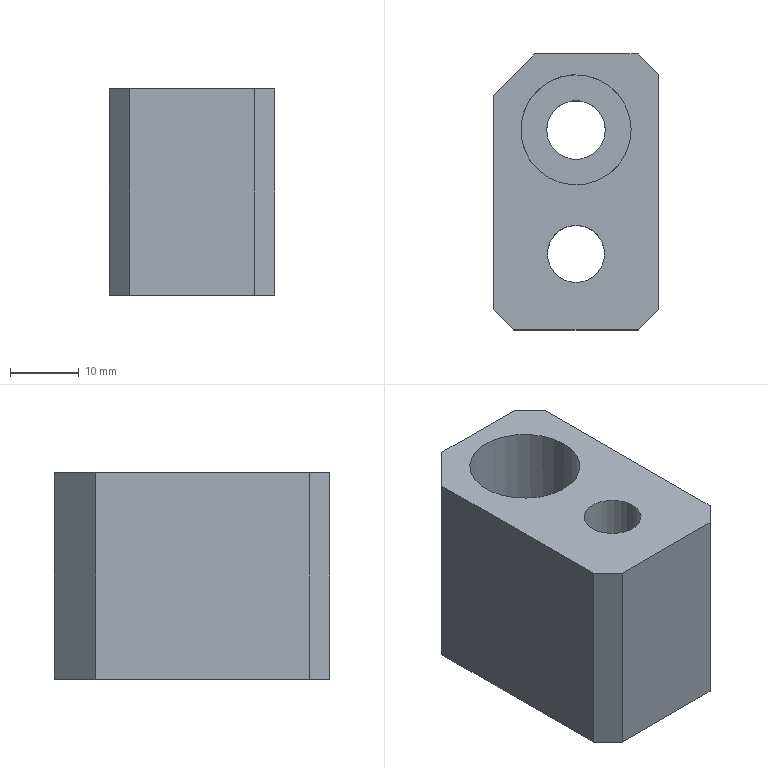Part | NX | features LIN_SOLID_COLOR 2 | 1 solid | 14 faces | box 24 x 40 x 30 mm | volume 22365 mm3 | plane 11 | cylinder 3 | commonest cylinder face diameters 8.3 x1 8.5 x1 16 x1
STEP:
#1=CARTESIAN_POINT('',(-225.,-65.,-31.5));
#2=VERTEX_POINT('',#1);
#3=CARTESIAN_POINT('',(-225.,-96.,-31.5));
#4=VERTEX_POINT('',#3);
#5=CARTESIAN_POINT('',(-225.,-81.,-31.5));
#6=DIRECTION('',(0.,-1.,0.));
#7=VECTOR('',#6,1000.);
#8=LINE('',#5,#7);
#9=EDGE_CURVE('',#2,#4,#8,.T.);
#10=ORIENTED_EDGE('',*,*,#9,.F.);
#11=CARTESIAN_POINT('',(-219.,-59.,-31.5));
#12=VERTEX_POINT('',#11);
#13=CARTESIAN_POINT('',(-227.,-67.,-31.5));
#14=DIRECTION('',(-0.7071,-0.7071,0.));
#15=VECTOR('',#14,1000.);
#16=LINE('',#13,#15);
#17=EDGE_CURVE('',#2,#12,#16,.F.);
#18=ORIENTED_EDGE('',*,*,#17,.T.);
#19=CARTESIAN_POINT('',(-204.,-59.,-31.5));
#20=VERTEX_POINT('',#19);
#21=CARTESIAN_POINT('',(-213.,-59.,-31.5));
#22=DIRECTION('',(-1.,0.,0.));
#23=VECTOR('',#22,1000.);
#24=LINE('',#21,#23);
#25=EDGE_CURVE('',#20,#12,#24,.T.);
#26=ORIENTED_EDGE('',*,*,#25,.F.);
#27=CARTESIAN_POINT('',(-201.,-62.,-31.5));
#28=VERTEX_POINT('',#27);
#29=CARTESIAN_POINT('',(-197.5,-65.5,-31.5));
#30=DIRECTION('',(-0.7071,0.7071,0.));
#31=VECTOR('',#30,1000.);
#32=LINE('',#29,#31);
#33=EDGE_CURVE('',#20,#28,#32,.F.);
#34=ORIENTED_EDGE('',*,*,#33,.T.);
#35=CARTESIAN_POINT('',(-201.,-96.,-31.5));
#36=VERTEX_POINT('',#35);
#37=CARTESIAN_POINT('',(-201.,-81.,-31.5));
#38=DIRECTION('',(0.,1.,0.));
#39=VECTOR('',#38,1000.);
#40=LINE('',#37,#39);
#41=EDGE_CURVE('',#36,#28,#40,.T.);
#42=ORIENTED_EDGE('',*,*,#41,.F.);
#43=CARTESIAN_POINT('',(-204.,-99.,-31.5));
#44=VERTEX_POINT('',#43);
#45=CARTESIAN_POINT('',(-199.5,-94.5,-31.5));
#46=DIRECTION('',(0.7071,0.7071,0.));
#47=VECTOR('',#46,1000.);
#48=LINE('',#45,#47);
#49=EDGE_CURVE('',#36,#44,#48,.F.);
#50=ORIENTED_EDGE('',*,*,#49,.T.);
#51=CARTESIAN_POINT('',(-222.,-99.,-31.5));
#52=VERTEX_POINT('',#51);
#53=CARTESIAN_POINT('',(-213.,-99.,-31.5));
#54=DIRECTION('',(1.,0.,0.));
#55=VECTOR('',#54,1000.);
#56=LINE('',#53,#55);
#57=EDGE_CURVE('',#52,#44,#56,.T.);
#58=ORIENTED_EDGE('',*,*,#57,.F.);
#59=CARTESIAN_POINT('',(-226.5,-94.5,-31.5));
#60=DIRECTION('',(0.7071,-0.7071,0.));
#61=VECTOR('',#60,1000.);
#62=LINE('',#59,#61);
#63=EDGE_CURVE('',#52,#4,#62,.F.);
#64=ORIENTED_EDGE('',*,*,#63,.T.);
#65=EDGE_LOOP('',(#10,#18,#26,#34,#42,#50,#58,#64));
#66=FACE_BOUND('',#65,.T.);
#67=CARTESIAN_POINT('',(-208.85,-88.,-31.5));
#68=VERTEX_POINT('',#67);
#69=CARTESIAN_POINT('',(-213.,-88.,-31.5));
#70=DIRECTION('',(0.,0.,-1.));
#71=DIRECTION('',(1.,0.,0.));
#72=AXIS2_PLACEMENT_3D('',#69,#70,#71);
#73=CIRCLE('',#72,4.15);
#74=EDGE_CURVE('',#68,#68,#73,.T.);
#75=ORIENTED_EDGE('',*,*,#74,.F.);
#76=EDGE_LOOP('',(#75));
#77=FACE_BOUND('',#76,.T.);
#78=CARTESIAN_POINT('',(-217.25,-70.,-31.5));
#79=VERTEX_POINT('',#78);
#80=CARTESIAN_POINT('',(-213.,-70.,-31.5));
#81=DIRECTION('',(0.,0.,-1.));
#82=DIRECTION('',(-1.,0.,0.));
#83=AXIS2_PLACEMENT_3D('',#80,#81,#82);
#84=CIRCLE('',#83,4.25);
#85=EDGE_CURVE('',#79,#79,#84,.F.);
#86=ORIENTED_EDGE('',*,*,#85,.T.);
#87=EDGE_LOOP('',(#86));
#88=FACE_BOUND('',#87,.T.);
#89=CARTESIAN_POINT('',(-213.,-81.,-31.5));
#90=DIRECTION('',(0.,0.,-1.));
#91=DIRECTION('',(0.,-1.,0.));
#92=AXIS2_PLACEMENT_3D('',#89,#90,#91);
#93=PLANE('',#92);
#94=ADVANCED_FACE('',(#66,#77,#88),#93,.T.);
#95=CARTESIAN_POINT('',(-205.,-70.,-1.5));
#96=VERTEX_POINT('',#95);
#97=CARTESIAN_POINT('',(-213.,-70.,-1.5));
#98=DIRECTION('',(0.,0.,1.));
#99=DIRECTION('',(1.,0.,0.));
#100=AXIS2_PLACEMENT_3D('',#97,#98,#99);
#101=CIRCLE('',#100,8.);
#102=EDGE_CURVE('',#96,#96,#101,.T.);
#103=ORIENTED_EDGE('',*,*,#102,.F.);
#104=EDGE_LOOP('',(#103));
#105=FACE_BOUND('',#104,.T.);
#106=CARTESIAN_POINT('',(-217.15,-88.,-1.5));
#107=VERTEX_POINT('',#106);
#108=CARTESIAN_POINT('',(-213.,-88.,-1.5));
#109=DIRECTION('',(0.,0.,1.));
#110=DIRECTION('',(-1.,0.,0.));
#111=AXIS2_PLACEMENT_3D('',#108,#109,#110);
#112=CIRCLE('',#111,4.15);
#113=EDGE_CURVE('',#107,#107,#112,.T.);
#114=ORIENTED_EDGE('',*,*,#113,.F.);
#115=EDGE_LOOP('',(#114));
#116=FACE_BOUND('',#115,.T.);
#117=CARTESIAN_POINT('',(-219.,-59.,-1.5));
#118=VERTEX_POINT('',#117);
#119=CARTESIAN_POINT('',(-204.,-59.,-1.5));
#120=VERTEX_POINT('',#119);
#121=CARTESIAN_POINT('',(-213.,-59.,-1.5));
#122=DIRECTION('',(1.,0.,0.));
#123=VECTOR('',#122,1000.);
#124=LINE('',#121,#123);
#125=EDGE_CURVE('',#118,#120,#124,.T.);
#126=ORIENTED_EDGE('',*,*,#125,.F.);
#127=CARTESIAN_POINT('',(-225.,-65.,-1.5));
#128=VERTEX_POINT('',#127);
#129=CARTESIAN_POINT('',(-227.,-67.,-1.5));
#130=DIRECTION('',(0.7071,0.7071,0.));
#131=VECTOR('',#130,1000.);
#132=LINE('',#129,#131);
#133=EDGE_CURVE('',#118,#128,#132,.F.);
#134=ORIENTED_EDGE('',*,*,#133,.T.);
#135=CARTESIAN_POINT('',(-225.,-96.,-1.5));
#136=VERTEX_POINT('',#135);
#137=CARTESIAN_POINT('',(-225.,-81.,-1.5));
#138=DIRECTION('',(0.,1.,0.));
#139=VECTOR('',#138,1000.);
#140=LINE('',#137,#139);
#141=EDGE_CURVE('',#136,#128,#140,.T.);
#142=ORIENTED_EDGE('',*,*,#141,.F.);
#143=CARTESIAN_POINT('',(-222.,-99.,-1.5));
#144=VERTEX_POINT('',#143);
#145=CARTESIAN_POINT('',(-226.5,-94.5,-1.5));
#146=DIRECTION('',(-0.7071,0.7071,0.));
#147=VECTOR('',#146,1000.);
#148=LINE('',#145,#147);
#149=EDGE_CURVE('',#136,#144,#148,.F.);
#150=ORIENTED_EDGE('',*,*,#149,.T.);
#151=CARTESIAN_POINT('',(-204.,-99.,-1.5));
#152=VERTEX_POINT('',#151);
#153=CARTESIAN_POINT('',(-213.,-99.,-1.5));
#154=DIRECTION('',(-1.,0.,0.));
#155=VECTOR('',#154,1000.);
#156=LINE('',#153,#155);
#157=EDGE_CURVE('',#152,#144,#156,.T.);
#158=ORIENTED_EDGE('',*,*,#157,.F.);
#159=CARTESIAN_POINT('',(-201.,-96.,-1.5));
#160=VERTEX_POINT('',#159);
#161=CARTESIAN_POINT('',(-199.5,-94.5,-1.5));
#162=DIRECTION('',(-0.7071,-0.7071,0.));
#163=VECTOR('',#162,1000.);
#164=LINE('',#161,#163);
#165=EDGE_CURVE('',#152,#160,#164,.F.);
#166=ORIENTED_EDGE('',*,*,#165,.T.);
#167=CARTESIAN_POINT('',(-201.,-62.,-1.5));
#168=VERTEX_POINT('',#167);
#169=CARTESIAN_POINT('',(-201.,-81.,-1.5));
#170=DIRECTION('',(0.,-1.,0.));
#171=VECTOR('',#170,1000.);
#172=LINE('',#169,#171);
#173=EDGE_CURVE('',#168,#160,#172,.T.);
#174=ORIENTED_EDGE('',*,*,#173,.F.);
#175=CARTESIAN_POINT('',(-197.5,-65.5,-1.5));
#176=DIRECTION('',(0.7071,-0.7071,0.));
#177=VECTOR('',#176,1000.);
#178=LINE('',#175,#177);
#179=EDGE_CURVE('',#168,#120,#178,.F.);
#180=ORIENTED_EDGE('',*,*,#179,.T.);
#181=EDGE_LOOP('',(#126,#134,#142,#150,#158,#166,#174,#180));
#182=FACE_BOUND('',#181,.T.);
#183=CARTESIAN_POINT('',(-213.,-81.,-1.5));
#184=DIRECTION('',(0.,0.,1.));
#185=DIRECTION('',(0.,1.,0.));
#186=AXIS2_PLACEMENT_3D('',#183,#184,#185);
#187=PLANE('',#186);
#188=ADVANCED_FACE('',(#105,#116,#182),#187,.T.);
#189=ORIENTED_EDGE('',*,*,#41,.T.);
#190=CARTESIAN_POINT('',(-201.,-62.,-31.5));
#191=DIRECTION('',(0.,0.,1.));
#192=VECTOR('',#191,1000.);
#193=LINE('',#190,#192);
#194=EDGE_CURVE('',#28,#168,#193,.T.);
#195=ORIENTED_EDGE('',*,*,#194,.T.);
#196=ORIENTED_EDGE('',*,*,#173,.T.);
#197=CARTESIAN_POINT('',(-201.,-96.,-31.5));
#198=DIRECTION('',(0.,0.,-1.));
#199=VECTOR('',#198,1000.);
#200=LINE('',#197,#199);
#201=EDGE_CURVE('',#160,#36,#200,.T.);
#202=ORIENTED_EDGE('',*,*,#201,.T.);
#203=EDGE_LOOP('',(#189,#195,#196,#202));
#204=FACE_BOUND('',#203,.T.);
#205=CARTESIAN_POINT('',(-201.,-81.,-31.5));
#206=DIRECTION('',(1.,0.,0.));
#207=DIRECTION('',(0.,0.,-1.));
#208=AXIS2_PLACEMENT_3D('',#205,#206,#207);
#209=PLANE('',#208);
#210=ADVANCED_FACE('',(#204),#209,.T.);
#211=ORIENTED_EDGE('',*,*,#157,.T.);
#212=CARTESIAN_POINT('',(-222.,-99.,-31.5));
#213=DIRECTION('',(0.,0.,-1.));
#214=VECTOR('',#213,1000.);
#215=LINE('',#212,#214);
#216=EDGE_CURVE('',#144,#52,#215,.T.);
#217=ORIENTED_EDGE('',*,*,#216,.T.);
#218=ORIENTED_EDGE('',*,*,#57,.T.);
#219=CARTESIAN_POINT('',(-204.,-99.,-31.5));
#220=DIRECTION('',(0.,0.,1.));
#221=VECTOR('',#220,1000.);
#222=LINE('',#219,#221);
#223=EDGE_CURVE('',#44,#152,#222,.T.);
#224=ORIENTED_EDGE('',*,*,#223,.T.);
#225=EDGE_LOOP('',(#211,#217,#218,#224));
#226=FACE_BOUND('',#225,.T.);
#227=CARTESIAN_POINT('',(-213.,-99.,-31.5));
#228=DIRECTION('',(0.,-1.,0.));
#229=DIRECTION('',(0.,0.,1.));
#230=AXIS2_PLACEMENT_3D('',#227,#228,#229);
#231=PLANE('',#230);
#232=ADVANCED_FACE('',(#226),#231,.T.);
#233=ORIENTED_EDGE('',*,*,#141,.T.);
#234=CARTESIAN_POINT('',(-225.,-65.,-31.5));
#235=DIRECTION('',(0.,0.,-1.));
#236=VECTOR('',#235,1000.);
#237=LINE('',#234,#236);
#238=EDGE_CURVE('',#128,#2,#237,.T.);
#239=ORIENTED_EDGE('',*,*,#238,.T.);
#240=ORIENTED_EDGE('',*,*,#9,.T.);
#241=CARTESIAN_POINT('',(-225.,-96.,-31.5));
#242=DIRECTION('',(0.,0.,1.));
#243=VECTOR('',#242,1000.);
#244=LINE('',#241,#243);
#245=EDGE_CURVE('',#4,#136,#244,.T.);
#246=ORIENTED_EDGE('',*,*,#245,.T.);
#247=EDGE_LOOP('',(#233,#239,#240,#246));
#248=FACE_BOUND('',#247,.T.);
#249=CARTESIAN_POINT('',(-225.,-81.,-31.5));
#250=DIRECTION('',(-1.,0.,0.));
#251=DIRECTION('',(0.,0.,1.));
#252=AXIS2_PLACEMENT_3D('',#249,#250,#251);
#253=PLANE('',#252);
#254=ADVANCED_FACE('',(#248),#253,.T.);
#255=ORIENTED_EDGE('',*,*,#25,.T.);
#256=CARTESIAN_POINT('',(-219.,-59.,-31.5));
#257=DIRECTION('',(0.,0.,1.));
#258=VECTOR('',#257,1000.);
#259=LINE('',#256,#258);
#260=EDGE_CURVE('',#12,#118,#259,.T.);
#261=ORIENTED_EDGE('',*,*,#260,.T.);
#262=ORIENTED_EDGE('',*,*,#125,.T.);
#263=CARTESIAN_POINT('',(-204.,-59.,-31.5));
#264=DIRECTION('',(0.,0.,-1.));
#265=VECTOR('',#264,1000.);
#266=LINE('',#263,#265);
#267=EDGE_CURVE('',#120,#20,#266,.T.);
#268=ORIENTED_EDGE('',*,*,#267,.T.);
#269=EDGE_LOOP('',(#255,#261,#262,#268));
#270=FACE_BOUND('',#269,.T.);
#271=CARTESIAN_POINT('',(-213.,-59.,-31.5));
#272=DIRECTION('',(0.,1.,0.));
#273=DIRECTION('',(0.,0.,-1.));
#274=AXIS2_PLACEMENT_3D('',#271,#272,#273);
#275=PLANE('',#274);
#276=ADVANCED_FACE('',(#270),#275,.T.);
#277=ORIENTED_EDGE('',*,*,#113,.T.);
#278=EDGE_LOOP('',(#277));
#279=FACE_BOUND('',#278,.T.);
#280=ORIENTED_EDGE('',*,*,#74,.T.);
#281=EDGE_LOOP('',(#280));
#282=FACE_BOUND('',#281,.T.);
#283=CARTESIAN_POINT('',(-213.,-88.,-66.5));
#284=DIRECTION('',(0.,0.,1.));
#285=DIRECTION('',(0.,1.,0.));
#286=AXIS2_PLACEMENT_3D('',#283,#284,#285);
#287=CYLINDRICAL_SURFACE('',#286,4.15);
#288=ADVANCED_FACE('',(#279,#282),#287,.F.);
#289=CARTESIAN_POINT('',(-217.25,-70.,-16.5));
#290=VERTEX_POINT('',#289);
#291=CARTESIAN_POINT('',(-213.,-70.,-16.5));
#292=DIRECTION('',(0.,0.,-1.));
#293=DIRECTION('',(-1.,0.,0.));
#294=AXIS2_PLACEMENT_3D('',#291,#292,#293);
#295=CIRCLE('',#294,4.25);
#296=EDGE_CURVE('',#290,#290,#295,.F.);
#297=ORIENTED_EDGE('',*,*,#296,.T.);
#298=EDGE_LOOP('',(#297));
#299=FACE_BOUND('',#298,.T.);
#300=ORIENTED_EDGE('',*,*,#85,.F.);
#301=EDGE_LOOP('',(#300));
#302=FACE_BOUND('',#301,.T.);
#303=CARTESIAN_POINT('',(-213.,-70.,-31.5));
#304=DIRECTION('',(0.,0.,1.));
#305=DIRECTION('',(0.,1.,0.));
#306=AXIS2_PLACEMENT_3D('',#303,#304,#305);
#307=CYLINDRICAL_SURFACE('',#306,4.25);
#308=ADVANCED_FACE('',(#299,#302),#307,.F.);
#309=CARTESIAN_POINT('',(-221.,-70.,-16.5));
#310=VERTEX_POINT('',#309);
#311=CARTESIAN_POINT('',(-213.,-70.,-16.5));
#312=DIRECTION('',(0.,0.,-1.));
#313=DIRECTION('',(-1.,0.,0.));
#314=AXIS2_PLACEMENT_3D('',#311,#312,#313);
#315=CIRCLE('',#314,8.);
#316=EDGE_CURVE('',#310,#310,#315,.T.);
#317=ORIENTED_EDGE('',*,*,#316,.F.);
#318=EDGE_LOOP('',(#317));
#319=FACE_BOUND('',#318,.T.);
#320=ORIENTED_EDGE('',*,*,#296,.F.);
#321=EDGE_LOOP('',(#320));
#322=FACE_BOUND('',#321,.T.);
#323=CARTESIAN_POINT('',(-213.,-70.,-16.5));
#324=DIRECTION('',(0.,0.,-1.));
#325=DIRECTION('',(0.,-1.,0.));
#326=AXIS2_PLACEMENT_3D('',#323,#324,#325);
#327=PLANE('',#326);
#328=ADVANCED_FACE('',(#319,#322),#327,.F.);
#329=ORIENTED_EDGE('',*,*,#102,.T.);
#330=EDGE_LOOP('',(#329));
#331=FACE_BOUND('',#330,.T.);
#332=ORIENTED_EDGE('',*,*,#316,.T.);
#333=EDGE_LOOP('',(#332));
#334=FACE_BOUND('',#333,.T.);
#335=CARTESIAN_POINT('',(-213.,-70.,-11.5));
#336=DIRECTION('',(0.,0.,1.));
#337=DIRECTION('',(0.,1.,0.));
#338=AXIS2_PLACEMENT_3D('',#335,#336,#337);
#339=CYLINDRICAL_SURFACE('',#338,8.);
#340=ADVANCED_FACE('',(#331,#334),#339,.F.);
#341=ORIENTED_EDGE('',*,*,#33,.F.);
#342=ORIENTED_EDGE('',*,*,#267,.F.);
#343=ORIENTED_EDGE('',*,*,#179,.F.);
#344=ORIENTED_EDGE('',*,*,#194,.F.);
#345=EDGE_LOOP('',(#341,#342,#343,#344));
#346=FACE_BOUND('',#345,.T.);
#347=CARTESIAN_POINT('',(-201.,-62.,-31.5));
#348=DIRECTION('',(-0.7071,-0.7071,0.));
#349=DIRECTION('',(0.,0.,1.));
#350=AXIS2_PLACEMENT_3D('',#347,#348,#349);
#351=PLANE('',#350);
#352=ADVANCED_FACE('',(#346),#351,.F.);
#353=ORIENTED_EDGE('',*,*,#63,.F.);
#354=ORIENTED_EDGE('',*,*,#216,.F.);
#355=ORIENTED_EDGE('',*,*,#149,.F.);
#356=ORIENTED_EDGE('',*,*,#245,.F.);
#357=EDGE_LOOP('',(#353,#354,#355,#356));
#358=FACE_BOUND('',#357,.T.);
#359=CARTESIAN_POINT('',(-225.,-96.,-31.5));
#360=DIRECTION('',(0.7071,0.7071,0.));
#361=DIRECTION('',(0.,0.,1.));
#362=AXIS2_PLACEMENT_3D('',#359,#360,#361);
#363=PLANE('',#362);
#364=ADVANCED_FACE('',(#358),#363,.F.);
#365=ORIENTED_EDGE('',*,*,#49,.F.);
#366=ORIENTED_EDGE('',*,*,#201,.F.);
#367=ORIENTED_EDGE('',*,*,#165,.F.);
#368=ORIENTED_EDGE('',*,*,#223,.F.);
#369=EDGE_LOOP('',(#365,#366,#367,#368));
#370=FACE_BOUND('',#369,.T.);
#371=CARTESIAN_POINT('',(-204.,-99.,-31.5));
#372=DIRECTION('',(-0.7071,0.7071,0.));
#373=DIRECTION('',(0.,0.,1.));
#374=AXIS2_PLACEMENT_3D('',#371,#372,#373);
#375=PLANE('',#374);
#376=ADVANCED_FACE('',(#370),#375,.F.);
#377=ORIENTED_EDGE('',*,*,#17,.F.);
#378=ORIENTED_EDGE('',*,*,#238,.F.);
#379=ORIENTED_EDGE('',*,*,#133,.F.);
#380=ORIENTED_EDGE('',*,*,#260,.F.);
#381=EDGE_LOOP('',(#377,#378,#379,#380));
#382=FACE_BOUND('',#381,.T.);
#383=CARTESIAN_POINT('',(-219.,-59.,-31.5));
#384=DIRECTION('',(0.7071,-0.7071,0.));
#385=DIRECTION('',(0.,0.,1.));
#386=AXIS2_PLACEMENT_3D('',#383,#384,#385);
#387=PLANE('',#386);
#388=ADVANCED_FACE('',(#382),#387,.F.);
#389=CLOSED_SHELL('',(#94,#188,#210,#232,#254,#276,#288,#308,#328,#340,#352,#364,#376,#388));
#390=MANIFOLD_SOLID_BREP('',#389);
#391=(LENGTH_UNIT()NAMED_UNIT(*)SI_UNIT(.MILLI.,.METRE.));
#392=UNCERTAINTY_MEASURE_WITH_UNIT(LENGTH_MEASURE(0.00001),#391,'','');
#393=(NAMED_UNIT(*)PLANE_ANGLE_UNIT()SI_UNIT($,.RADIAN.));
#394=(NAMED_UNIT(*)SI_UNIT($,.STERADIAN.)SOLID_ANGLE_UNIT());
#395=(GEOMETRIC_REPRESENTATION_CONTEXT(3)GLOBAL_UNCERTAINTY_ASSIGNED_CONTEXT((#392))GLOBAL_UNIT_ASSIGNED_CONTEXT((#391,#393,#394))REPRESENTATION_CONTEXT('',''));
#396=ADVANCED_BREP_SHAPE_REPRESENTATION('',(#390),#395);